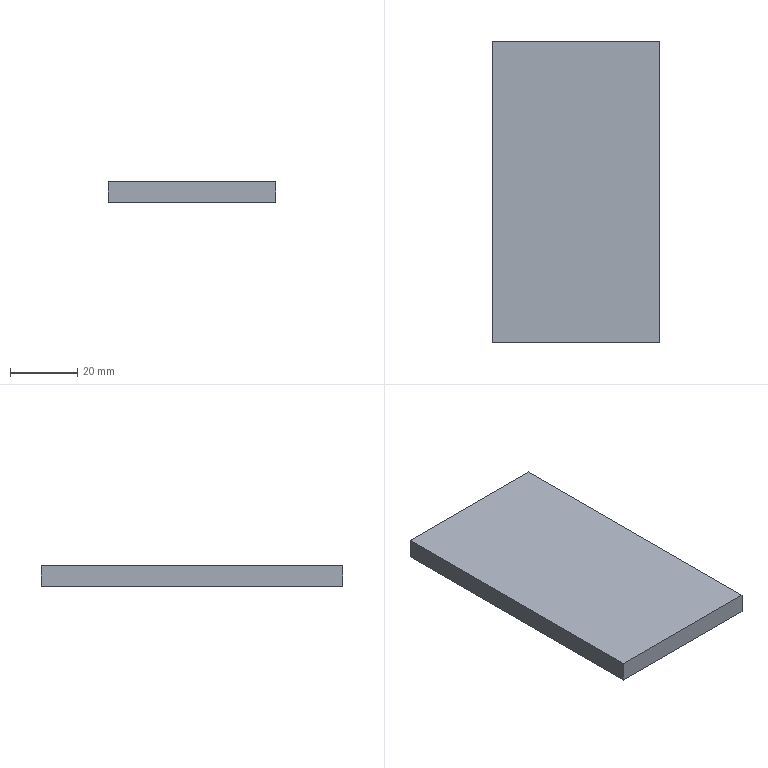Part | SolidWorks | features FlatPattern 1, SMBaseFlange 1, SheetMetal 1 | 1 solid | 6 faces | box 50 x 90 x 6 mm | volume 27000 mm3 | plane 6
STEP:
#1=CARTESIAN_POINT('',(-50.,0.,0.));
#2=VERTEX_POINT('',#1);
#3=CARTESIAN_POINT('',(0.,0.,0.));
#4=VERTEX_POINT('',#3);
#5=CARTESIAN_POINT('',(-50.,0.,0.));
#6=DIRECTION('',(1.,0.,0.));
#7=VECTOR('',#6,1000.);
#8=LINE('',#5,#7);
#9=EDGE_CURVE('',#2,#4,#8,.T.);
#10=ORIENTED_EDGE('',*,*,#9,.T.);
#11=CARTESIAN_POINT('',(0.,0.,6.));
#12=VERTEX_POINT('',#11);
#13=CARTESIAN_POINT('',(0.,0.,6.));
#14=DIRECTION('',(0.,0.,-1.));
#15=VECTOR('',#14,1000.);
#16=LINE('',#13,#15);
#17=EDGE_CURVE('',#12,#4,#16,.T.);
#18=ORIENTED_EDGE('',*,*,#17,.F.);
#19=CARTESIAN_POINT('',(-50.,0.,6.));
#20=VERTEX_POINT('',#19);
#21=CARTESIAN_POINT('',(-50.,0.,6.));
#22=DIRECTION('',(1.,0.,0.));
#23=VECTOR('',#22,1000.);
#24=LINE('',#21,#23);
#25=EDGE_CURVE('',#20,#12,#24,.T.);
#26=ORIENTED_EDGE('',*,*,#25,.F.);
#27=CARTESIAN_POINT('',(-50.,0.,6.));
#28=DIRECTION('',(0.,0.,-1.));
#29=VECTOR('',#28,1000.);
#30=LINE('',#27,#29);
#31=EDGE_CURVE('',#20,#2,#30,.T.);
#32=ORIENTED_EDGE('',*,*,#31,.T.);
#33=EDGE_LOOP('',(#10,#18,#26,#32));
#34=FACE_OUTER_BOUND('',#33,.T.);
#35=CARTESIAN_POINT('',(-50.,0.,6.));
#36=DIRECTION('',(0.,1.,0.));
#37=DIRECTION('',(0.,0.,1.));
#38=AXIS2_PLACEMENT_3D('',#35,#36,#37);
#39=PLANE('',#38);
#40=ADVANCED_FACE('',(#34),#39,.F.);
#41=CARTESIAN_POINT('',(0.,90.,0.));
#42=VERTEX_POINT('',#41);
#43=CARTESIAN_POINT('',(0.,0.,0.));
#44=DIRECTION('',(0.,1.,0.));
#45=VECTOR('',#44,1000.);
#46=LINE('',#43,#45);
#47=EDGE_CURVE('',#4,#42,#46,.T.);
#48=ORIENTED_EDGE('',*,*,#47,.T.);
#49=CARTESIAN_POINT('',(0.,90.,6.));
#50=VERTEX_POINT('',#49);
#51=CARTESIAN_POINT('',(0.,90.,6.));
#52=DIRECTION('',(0.,0.,-1.));
#53=VECTOR('',#52,1000.);
#54=LINE('',#51,#53);
#55=EDGE_CURVE('',#50,#42,#54,.T.);
#56=ORIENTED_EDGE('',*,*,#55,.F.);
#57=CARTESIAN_POINT('',(0.,0.,6.));
#58=DIRECTION('',(0.,1.,0.));
#59=VECTOR('',#58,1000.);
#60=LINE('',#57,#59);
#61=EDGE_CURVE('',#12,#50,#60,.T.);
#62=ORIENTED_EDGE('',*,*,#61,.F.);
#63=ORIENTED_EDGE('',*,*,#17,.T.);
#64=EDGE_LOOP('',(#48,#56,#62,#63));
#65=FACE_OUTER_BOUND('',#64,.T.);
#66=CARTESIAN_POINT('',(0.,0.,6.));
#67=DIRECTION('',(-1.,0.,0.));
#68=DIRECTION('',(0.,0.,1.));
#69=AXIS2_PLACEMENT_3D('',#66,#67,#68);
#70=PLANE('',#69);
#71=ADVANCED_FACE('',(#65),#70,.F.);
#72=CARTESIAN_POINT('',(-50.,90.,0.));
#73=VERTEX_POINT('',#72);
#74=CARTESIAN_POINT('',(0.,90.,0.));
#75=DIRECTION('',(-1.,0.,0.));
#76=VECTOR('',#75,1000.);
#77=LINE('',#74,#76);
#78=EDGE_CURVE('',#42,#73,#77,.T.);
#79=ORIENTED_EDGE('',*,*,#78,.T.);
#80=CARTESIAN_POINT('',(-50.,90.,6.));
#81=VERTEX_POINT('',#80);
#82=CARTESIAN_POINT('',(-50.,90.,6.));
#83=DIRECTION('',(0.,0.,-1.));
#84=VECTOR('',#83,1000.);
#85=LINE('',#82,#84);
#86=EDGE_CURVE('',#81,#73,#85,.T.);
#87=ORIENTED_EDGE('',*,*,#86,.F.);
#88=CARTESIAN_POINT('',(0.,90.,6.));
#89=DIRECTION('',(-1.,0.,0.));
#90=VECTOR('',#89,1000.);
#91=LINE('',#88,#90);
#92=EDGE_CURVE('',#50,#81,#91,.T.);
#93=ORIENTED_EDGE('',*,*,#92,.F.);
#94=ORIENTED_EDGE('',*,*,#55,.T.);
#95=EDGE_LOOP('',(#79,#87,#93,#94));
#96=FACE_OUTER_BOUND('',#95,.T.);
#97=CARTESIAN_POINT('',(0.,90.,6.));
#98=DIRECTION('',(0.,-1.,0.));
#99=DIRECTION('',(0.,0.,-1.));
#100=AXIS2_PLACEMENT_3D('',#97,#98,#99);
#101=PLANE('',#100);
#102=ADVANCED_FACE('',(#96),#101,.F.);
#103=CARTESIAN_POINT('',(-50.,90.,0.));
#104=DIRECTION('',(0.,-1.,0.));
#105=VECTOR('',#104,1000.);
#106=LINE('',#103,#105);
#107=EDGE_CURVE('',#73,#2,#106,.T.);
#108=ORIENTED_EDGE('',*,*,#107,.T.);
#109=ORIENTED_EDGE('',*,*,#31,.F.);
#110=CARTESIAN_POINT('',(-50.,90.,6.));
#111=DIRECTION('',(0.,-1.,0.));
#112=VECTOR('',#111,1000.);
#113=LINE('',#110,#112);
#114=EDGE_CURVE('',#81,#20,#113,.T.);
#115=ORIENTED_EDGE('',*,*,#114,.F.);
#116=ORIENTED_EDGE('',*,*,#86,.T.);
#117=EDGE_LOOP('',(#108,#109,#115,#116));
#118=FACE_OUTER_BOUND('',#117,.T.);
#119=CARTESIAN_POINT('',(-50.,90.,6.));
#120=DIRECTION('',(1.,0.,0.));
#121=DIRECTION('',(0.,1.,0.));
#122=AXIS2_PLACEMENT_3D('',#119,#120,#121);
#123=PLANE('',#122);
#124=ADVANCED_FACE('',(#118),#123,.F.);
#125=ORIENTED_EDGE('',*,*,#25,.T.);
#126=ORIENTED_EDGE('',*,*,#61,.T.);
#127=ORIENTED_EDGE('',*,*,#92,.T.);
#128=ORIENTED_EDGE('',*,*,#114,.T.);
#129=EDGE_LOOP('',(#125,#126,#127,#128));
#130=FACE_OUTER_BOUND('',#129,.T.);
#131=CARTESIAN_POINT('',(0.,0.,6.));
#132=DIRECTION('',(0.,0.,1.));
#133=DIRECTION('',(1.,0.,0.));
#134=AXIS2_PLACEMENT_3D('',#131,#132,#133);
#135=PLANE('',#134);
#136=ADVANCED_FACE('',(#130),#135,.T.);
#137=ORIENTED_EDGE('',*,*,#9,.F.);
#138=ORIENTED_EDGE('',*,*,#107,.F.);
#139=ORIENTED_EDGE('',*,*,#78,.F.);
#140=ORIENTED_EDGE('',*,*,#47,.F.);
#141=EDGE_LOOP('',(#137,#138,#139,#140));
#142=FACE_OUTER_BOUND('',#141,.T.);
#143=CARTESIAN_POINT('',(0.,0.,0.));
#144=DIRECTION('',(0.,0.,1.));
#145=DIRECTION('',(1.,0.,0.));
#146=AXIS2_PLACEMENT_3D('',#143,#144,#145);
#147=PLANE('',#146);
#148=ADVANCED_FACE('',(#142),#147,.F.);
#149=CLOSED_SHELL('',(#40,#71,#102,#124,#136,#148));
#150=MANIFOLD_SOLID_BREP('',#149);
#151=CARTESIAN_POINT('',(0.,0.,0.));
#152=DIRECTION('',(0.,0.,1.));
#153=DIRECTION('',(1.,0.,0.));
#154=AXIS2_PLACEMENT_3D('',#151,#152,#153);
#155=(LENGTH_UNIT()NAMED_UNIT(*)SI_UNIT(.MILLI.,.METRE.));
#156=UNCERTAINTY_MEASURE_WITH_UNIT(LENGTH_MEASURE(0.00001),#155,'','');
#157=(NAMED_UNIT(*)PLANE_ANGLE_UNIT()SI_UNIT($,.RADIAN.));
#158=(NAMED_UNIT(*)SI_UNIT($,.STERADIAN.)SOLID_ANGLE_UNIT());
#159=(GEOMETRIC_REPRESENTATION_CONTEXT(3)GLOBAL_UNCERTAINTY_ASSIGNED_CONTEXT((#156))GLOBAL_UNIT_ASSIGNED_CONTEXT((#155,#157,#158))REPRESENTATION_CONTEXT('',''));
#160=ADVANCED_BREP_SHAPE_REPRESENTATION('',(#150,#154),#159);